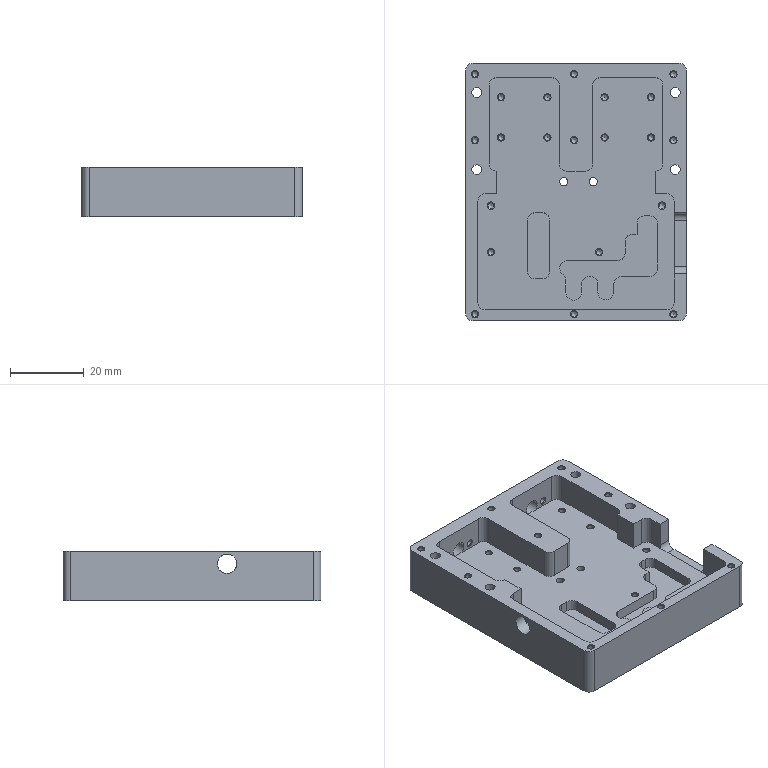Part | STEP file | VSWR protection cavity | 1 solid | 173 faces | box 60 x 70.12 x 13.5 mm | volume 30547 mm3 | cylinder 72 | plane 51 | cone 50 | commonest cylinder face diameters 4 x35 1.6 x25 2.7 x4 2.2 x2 4.1 x2 4.311 x2